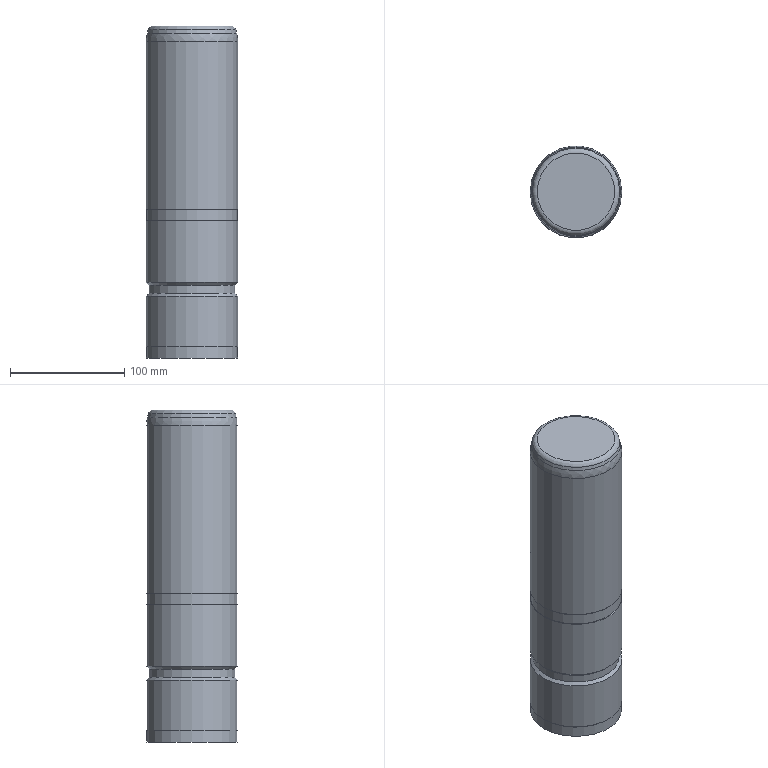Part | NX | features solid 2 | 1 solid | 16 faces | box 80 x 80 x 290 mm | volume 1446036 mm3 | cylinder 6 | plane 5 | cone 3 | torus 2 | commonest cylinder face diameters 80 x3 75 x1 79 x1 79.5 x1
STEP:
#1=CARTESIAN_POINT('',(1335.,-300.,-325.));
#2=VERTEX_POINT('',#1);
#3=CARTESIAN_POINT('',(1375.,-300.,-325.));
#4=DIRECTION('',(0.,0.,1.));
#5=DIRECTION('',(-1.,0.,0.));
#6=AXIS2_PLACEMENT_3D('',#3,#4,#5);
#7=CIRCLE('',#6,40.);
#8=EDGE_CURVE('',#2,#2,#7,.T.);
#9=ORIENTED_EDGE('',*,*,#8,.T.);
#10=EDGE_LOOP('',(#9));
#11=FACE_BOUND('',#10,.T.);
#12=CARTESIAN_POINT('',(1415.,-300.,-178.95));
#13=VERTEX_POINT('',#12);
#14=CARTESIAN_POINT('',(1375.,-300.,-178.95));
#15=DIRECTION('',(0.,0.,-1.));
#16=DIRECTION('',(1.,0.,0.));
#17=AXIS2_PLACEMENT_3D('',#14,#15,#16);
#18=CIRCLE('',#17,40.);
#19=EDGE_CURVE('',#13,#13,#18,.T.);
#20=ORIENTED_EDGE('',*,*,#19,.T.);
#21=EDGE_LOOP('',(#20));
#22=FACE_BOUND('',#21,.T.);
#23=CARTESIAN_POINT('',(1375.,-300.,-295.));
#24=DIRECTION('',(0.,0.,1.));
#25=DIRECTION('',(-1.,0.,0.));
#26=AXIS2_PLACEMENT_3D('',#23,#24,#25);
#27=CYLINDRICAL_SURFACE('',#26,40.);
#28=ADVANCED_FACE('',(#11,#22),#27,.T.);
#29=CARTESIAN_POINT('',(1412.5,-300.,-391.5));
#30=VERTEX_POINT('',#29);
#31=CARTESIAN_POINT('',(1375.,-300.,-391.5));
#32=DIRECTION('',(0.,0.,-1.));
#33=DIRECTION('',(1.,0.,0.));
#34=AXIS2_PLACEMENT_3D('',#31,#32,#33);
#35=CIRCLE('',#34,37.5);
#36=EDGE_CURVE('',#30,#30,#35,.T.);
#37=ORIENTED_EDGE('',*,*,#36,.F.);
#38=EDGE_LOOP('',(#37));
#39=FACE_BOUND('',#38,.T.);
#40=CARTESIAN_POINT('',(1335.,-300.,-389.));
#41=VERTEX_POINT('',#40);
#42=CARTESIAN_POINT('',(1375.,-300.,-389.));
#43=DIRECTION('',(0.,0.,1.));
#44=DIRECTION('',(-1.,0.,0.));
#45=AXIS2_PLACEMENT_3D('',#42,#43,#44);
#46=CIRCLE('',#45,40.);
#47=EDGE_CURVE('',#41,#41,#46,.T.);
#48=ORIENTED_EDGE('',*,*,#47,.F.);
#49=EDGE_LOOP('',(#48));
#50=FACE_BOUND('',#49,.T.);
#51=CARTESIAN_POINT('',(1375.,-300.,-391.5));
#52=DIRECTION('',(0.,0.,1.));
#53=DIRECTION('',(-1.,0.,0.));
#54=AXIS2_PLACEMENT_3D('',#51,#52,#53);
#55=CONICAL_SURFACE('',#54,37.5,0.7854);
#56=ADVANCED_FACE('',(#39,#50),#55,.T.);
#57=ORIENTED_EDGE('',*,*,#36,.T.);
#58=EDGE_LOOP('',(#57));
#59=FACE_BOUND('',#58,.T.);
#60=CARTESIAN_POINT('',(1412.5,-300.,-398.5));
#61=VERTEX_POINT('',#60);
#62=CARTESIAN_POINT('',(1375.,-300.,-398.5));
#63=DIRECTION('',(0.,0.,-1.));
#64=DIRECTION('',(1.,0.,0.));
#65=AXIS2_PLACEMENT_3D('',#62,#63,#64);
#66=CIRCLE('',#65,37.5);
#67=EDGE_CURVE('',#61,#61,#66,.T.);
#68=ORIENTED_EDGE('',*,*,#67,.F.);
#69=EDGE_LOOP('',(#68));
#70=FACE_BOUND('',#69,.T.);
#71=CARTESIAN_POINT('',(1375.,-300.,-398.5));
#72=DIRECTION('',(0.,0.,1.));
#73=DIRECTION('',(-1.,0.,0.));
#74=AXIS2_PLACEMENT_3D('',#71,#72,#73);
#75=CYLINDRICAL_SURFACE('',#74,37.5);
#76=ADVANCED_FACE('',(#59,#70),#75,.T.);
#77=CARTESIAN_POINT('',(1335.5,-300.,-335.));
#78=VERTEX_POINT('',#77);
#79=CARTESIAN_POINT('',(1375.,-300.,-335.));
#80=DIRECTION('',(0.,0.,1.));
#81=DIRECTION('',(-1.,0.,0.));
#82=AXIS2_PLACEMENT_3D('',#79,#80,#81);
#83=CIRCLE('',#82,39.5);
#84=EDGE_CURVE('',#78,#78,#83,.T.);
#85=ORIENTED_EDGE('',*,*,#84,.F.);
#86=EDGE_LOOP('',(#85));
#87=FACE_BOUND('',#86,.T.);
#88=CARTESIAN_POINT('',(1415.,-300.,-335.));
#89=VERTEX_POINT('',#88);
#90=CARTESIAN_POINT('',(1375.,-300.,-335.));
#91=DIRECTION('',(0.,0.,-1.));
#92=DIRECTION('',(1.,0.,0.));
#93=AXIS2_PLACEMENT_3D('',#90,#91,#92);
#94=CIRCLE('',#93,40.);
#95=EDGE_CURVE('',#89,#89,#94,.T.);
#96=ORIENTED_EDGE('',*,*,#95,.F.);
#97=EDGE_LOOP('',(#96));
#98=FACE_BOUND('',#97,.T.);
#99=CARTESIAN_POINT('',(1375.,-300.,-335.));
#100=DIRECTION('',(0.,0.,1.));
#101=DIRECTION('',(-1.,0.,0.));
#102=AXIS2_PLACEMENT_3D('',#99,#100,#101);
#103=PLANE('',#102);
#104=ADVANCED_FACE('',(#87,#98),#103,.T.);
#105=ORIENTED_EDGE('',*,*,#95,.T.);
#106=EDGE_LOOP('',(#105));
#107=FACE_BOUND('',#106,.T.);
#108=ORIENTED_EDGE('',*,*,#47,.T.);
#109=EDGE_LOOP('',(#108));
#110=FACE_BOUND('',#109,.T.);
#111=CARTESIAN_POINT('',(1375.,-300.,-389.));
#112=DIRECTION('',(0.,0.,1.));
#113=DIRECTION('',(-1.,0.,0.));
#114=AXIS2_PLACEMENT_3D('',#111,#112,#113);
#115=CYLINDRICAL_SURFACE('',#114,40.);
#116=ADVANCED_FACE('',(#107,#110),#115,.T.);
#117=CARTESIAN_POINT('',(1414.5,-300.,-325.));
#118=VERTEX_POINT('',#117);
#119=CARTESIAN_POINT('',(1375.,-300.,-325.));
#120=DIRECTION('',(0.,0.,-1.));
#121=DIRECTION('',(1.,0.,0.));
#122=AXIS2_PLACEMENT_3D('',#119,#120,#121);
#123=CIRCLE('',#122,39.5);
#124=EDGE_CURVE('',#118,#118,#123,.T.);
#125=ORIENTED_EDGE('',*,*,#124,.F.);
#126=EDGE_LOOP('',(#125));
#127=FACE_BOUND('',#126,.T.);
#128=ORIENTED_EDGE('',*,*,#8,.F.);
#129=EDGE_LOOP('',(#128));
#130=FACE_BOUND('',#129,.T.);
#131=CARTESIAN_POINT('',(1375.,-300.,-325.));
#132=DIRECTION('',(0.,0.,-1.));
#133=DIRECTION('',(1.,0.,0.));
#134=AXIS2_PLACEMENT_3D('',#131,#132,#133);
#135=PLANE('',#134);
#136=ADVANCED_FACE('',(#127,#130),#135,.T.);
#137=ORIENTED_EDGE('',*,*,#124,.T.);
#138=EDGE_LOOP('',(#137));
#139=FACE_BOUND('',#138,.T.);
#140=ORIENTED_EDGE('',*,*,#84,.T.);
#141=EDGE_LOOP('',(#140));
#142=FACE_BOUND('',#141,.T.);
#143=CARTESIAN_POINT('',(1375.,-300.,-335.));
#144=DIRECTION('',(0.,0.,1.));
#145=DIRECTION('',(-1.,0.,0.));
#146=AXIS2_PLACEMENT_3D('',#143,#144,#145);
#147=CYLINDRICAL_SURFACE('',#146,39.5);
#148=ADVANCED_FACE('',(#139,#142),#147,.T.);
#149=CARTESIAN_POINT('',(1414.75,-300.,-445.));
#150=VERTEX_POINT('',#149);
#151=CARTESIAN_POINT('',(1375.,-300.,-445.));
#152=DIRECTION('',(0.,0.,-1.));
#153=DIRECTION('',(1.,0.,0.));
#154=AXIS2_PLACEMENT_3D('',#151,#152,#153);
#155=CIRCLE('',#154,39.75);
#156=EDGE_CURVE('',#150,#150,#155,.T.);
#157=ORIENTED_EDGE('',*,*,#156,.F.);
#158=EDGE_LOOP('',(#157));
#159=FACE_BOUND('',#158,.T.);
#160=CARTESIAN_POINT('',(1335.,-300.,-445.));
#161=VERTEX_POINT('',#160);
#162=CARTESIAN_POINT('',(1375.,-300.,-445.));
#163=DIRECTION('',(0.,0.,1.));
#164=DIRECTION('',(-1.,0.,0.));
#165=AXIS2_PLACEMENT_3D('',#162,#163,#164);
#166=CIRCLE('',#165,40.);
#167=EDGE_CURVE('',#161,#161,#166,.T.);
#168=ORIENTED_EDGE('',*,*,#167,.F.);
#169=EDGE_LOOP('',(#168));
#170=FACE_BOUND('',#169,.T.);
#171=CARTESIAN_POINT('',(1375.,-300.,-445.));
#172=DIRECTION('',(0.,0.,-1.));
#173=DIRECTION('',(1.,0.,0.));
#174=AXIS2_PLACEMENT_3D('',#171,#172,#173);
#175=PLANE('',#174);
#176=ADVANCED_FACE('',(#159,#170),#175,.T.);
#177=CARTESIAN_POINT('',(1335.,-300.,-401.));
#178=VERTEX_POINT('',#177);
#179=CARTESIAN_POINT('',(1375.,-300.,-401.));
#180=DIRECTION('',(0.,0.,1.));
#181=DIRECTION('',(-1.,0.,0.));
#182=AXIS2_PLACEMENT_3D('',#179,#180,#181);
#183=CIRCLE('',#182,40.);
#184=EDGE_CURVE('',#178,#178,#183,.T.);
#185=ORIENTED_EDGE('',*,*,#184,.F.);
#186=EDGE_LOOP('',(#185));
#187=FACE_BOUND('',#186,.T.);
#188=ORIENTED_EDGE('',*,*,#167,.T.);
#189=EDGE_LOOP('',(#188));
#190=FACE_BOUND('',#189,.T.);
#191=CARTESIAN_POINT('',(1375.,-300.,-445.));
#192=DIRECTION('',(0.,0.,1.));
#193=DIRECTION('',(-1.,0.,0.));
#194=AXIS2_PLACEMENT_3D('',#191,#192,#193);
#195=CYLINDRICAL_SURFACE('',#194,40.);
#196=ADVANCED_FACE('',(#187,#190),#195,.T.);
#197=CARTESIAN_POINT('',(1335.25,-300.,-455.));
#198=VERTEX_POINT('',#197);
#199=CARTESIAN_POINT('',(1375.,-300.,-455.));
#200=DIRECTION('',(0.,0.,1.));
#201=DIRECTION('',(-1.,0.,0.));
#202=AXIS2_PLACEMENT_3D('',#199,#200,#201);
#203=CIRCLE('',#202,39.75);
#204=EDGE_CURVE('',#198,#198,#203,.T.);
#205=ORIENTED_EDGE('',*,*,#204,.F.);
#206=EDGE_LOOP('',(#205));
#207=FACE_BOUND('',#206,.T.);
#208=CARTESIAN_POINT('',(1375.,-300.,-455.));
#209=DIRECTION('',(0.,0.,-1.));
#210=DIRECTION('',(1.,0.,0.));
#211=AXIS2_PLACEMENT_3D('',#208,#209,#210);
#212=PLANE('',#211);
#213=ADVANCED_FACE('',(#207),#212,.T.);
#214=ORIENTED_EDGE('',*,*,#156,.T.);
#215=EDGE_LOOP('',(#214));
#216=FACE_BOUND('',#215,.T.);
#217=ORIENTED_EDGE('',*,*,#204,.T.);
#218=EDGE_LOOP('',(#217));
#219=FACE_BOUND('',#218,.T.);
#220=CARTESIAN_POINT('',(1375.,-300.,-455.));
#221=DIRECTION('',(0.,0.,1.));
#222=DIRECTION('',(-1.,0.,0.));
#223=AXIS2_PLACEMENT_3D('',#220,#221,#222);
#224=CYLINDRICAL_SURFACE('',#223,39.75);
#225=ADVANCED_FACE('',(#216,#219),#224,.T.);
#226=ORIENTED_EDGE('',*,*,#184,.T.);
#227=EDGE_LOOP('',(#226));
#228=FACE_BOUND('',#227,.T.);
#229=ORIENTED_EDGE('',*,*,#67,.T.);
#230=EDGE_LOOP('',(#229));
#231=FACE_BOUND('',#230,.T.);
#232=CARTESIAN_POINT('',(1375.,-300.,-398.5));
#233=DIRECTION('',(0.,0.,-1.));
#234=DIRECTION('',(1.,0.,0.));
#235=AXIS2_PLACEMENT_3D('',#232,#233,#234);
#236=CONICAL_SURFACE('',#235,37.5,0.7854);
#237=ADVANCED_FACE('',(#228,#231),#236,.T.);
#238=CARTESIAN_POINT('',(1341.132,-300.,-165.));
#239=VERTEX_POINT('',#238);
#240=CARTESIAN_POINT('',(1375.,-300.,-165.));
#241=DIRECTION('',(0.,0.,1.));
#242=DIRECTION('',(-1.,0.,0.));
#243=AXIS2_PLACEMENT_3D('',#240,#241,#242);
#244=CIRCLE('',#243,33.868);
#245=EDGE_CURVE('',#239,#239,#244,.T.);
#246=ORIENTED_EDGE('',*,*,#245,.T.);
#247=EDGE_LOOP('',(#246));
#248=FACE_BOUND('',#247,.T.);
#249=CARTESIAN_POINT('',(1375.,-300.,-165.));
#250=DIRECTION('',(0.,0.,1.));
#251=DIRECTION('',(-1.,0.,0.));
#252=AXIS2_PLACEMENT_3D('',#249,#250,#251);
#253=PLANE('',#252);
#254=ADVANCED_FACE('',(#248),#253,.T.);
#255=ORIENTED_EDGE('',*,*,#245,.F.);
#256=EDGE_LOOP('',(#255));
#257=FACE_BOUND('',#256,.T.);
#258=CARTESIAN_POINT('',(1336.786,-300.,-168.335));
#259=VERTEX_POINT('',#258);
#260=CARTESIAN_POINT('',(1375.,-300.,-168.335));
#261=DIRECTION('',(0.,0.,1.));
#262=DIRECTION('',(-1.,0.,0.));
#263=AXIS2_PLACEMENT_3D('',#260,#261,#262);
#264=CIRCLE('',#263,38.214);
#265=EDGE_CURVE('',#259,#259,#264,.F.);
#266=ORIENTED_EDGE('',*,*,#265,.F.);
#267=EDGE_LOOP('',(#266));
#268=FACE_BOUND('',#267,.T.);
#269=CARTESIAN_POINT('',(1375.,-300.,-169.5));
#270=DIRECTION('',(0.,0.,1.));
#271=DIRECTION('',(-1.,0.,0.));
#272=AXIS2_PLACEMENT_3D('',#269,#270,#271);
#273=TOROIDAL_SURFACE('',#272,33.868,4.5);
#274=ADVANCED_FACE('',(#257,#268),#273,.T.);
#275=ORIENTED_EDGE('',*,*,#265,.T.);
#276=EDGE_LOOP('',(#275));
#277=FACE_BOUND('',#276,.T.);
#278=CARTESIAN_POINT('',(1336.022,-300.,-171.185));
#279=VERTEX_POINT('',#278);
#280=CARTESIAN_POINT('',(1375.,-300.,-171.185));
#281=DIRECTION('',(0.,0.,1.));
#282=DIRECTION('',(-1.,0.,0.));
#283=AXIS2_PLACEMENT_3D('',#280,#281,#282);
#284=CIRCLE('',#283,38.978);
#285=EDGE_CURVE('',#279,#279,#284,.T.);
#286=ORIENTED_EDGE('',*,*,#285,.T.);
#287=EDGE_LOOP('',(#286));
#288=FACE_BOUND('',#287,.T.);
#289=CARTESIAN_POINT('',(1375.,-300.,-165.));
#290=DIRECTION('',(0.,0.,-1.));
#291=DIRECTION('',(1.,0.,0.));
#292=AXIS2_PLACEMENT_3D('',#289,#290,#291);
#293=CONICAL_SURFACE('',#292,37.321,0.2618);
#294=ADVANCED_FACE('',(#277,#288),#293,.T.);
#295=ORIENTED_EDGE('',*,*,#19,.F.);
#296=EDGE_LOOP('',(#295));
#297=FACE_BOUND('',#296,.T.);
#298=ORIENTED_EDGE('',*,*,#285,.F.);
#299=EDGE_LOOP('',(#298));
#300=FACE_BOUND('',#299,.T.);
#301=CARTESIAN_POINT('',(1375.,-300.,-178.95));
#302=DIRECTION('',(0.,0.,-1.));
#303=DIRECTION('',(1.,0.,0.));
#304=AXIS2_PLACEMENT_3D('',#301,#302,#303);
#305=DEGENERATE_TOROIDAL_SURFACE('',#304,10.,30.,.T.);
#306=ADVANCED_FACE('',(#297,#300),#305,.T.);
#307=CLOSED_SHELL('',(#28,#56,#76,#104,#116,#136,#148,#176,#196,#213,#225,#237,#254,#274,#294,#306));
#308=MANIFOLD_SOLID_BREP('',#307);
#309=(LENGTH_UNIT()NAMED_UNIT(*)SI_UNIT(.MILLI.,.METRE.));
#310=UNCERTAINTY_MEASURE_WITH_UNIT(LENGTH_MEASURE(0.00001),#309,'','');
#311=(NAMED_UNIT(*)PLANE_ANGLE_UNIT()SI_UNIT($,.RADIAN.));
#312=(NAMED_UNIT(*)SI_UNIT($,.STERADIAN.)SOLID_ANGLE_UNIT());
#313=(GEOMETRIC_REPRESENTATION_CONTEXT(3)GLOBAL_UNCERTAINTY_ASSIGNED_CONTEXT((#310))GLOBAL_UNIT_ASSIGNED_CONTEXT((#309,#311,#312))REPRESENTATION_CONTEXT('',''));
#314=ADVANCED_BREP_SHAPE_REPRESENTATION('',(#308),#313);